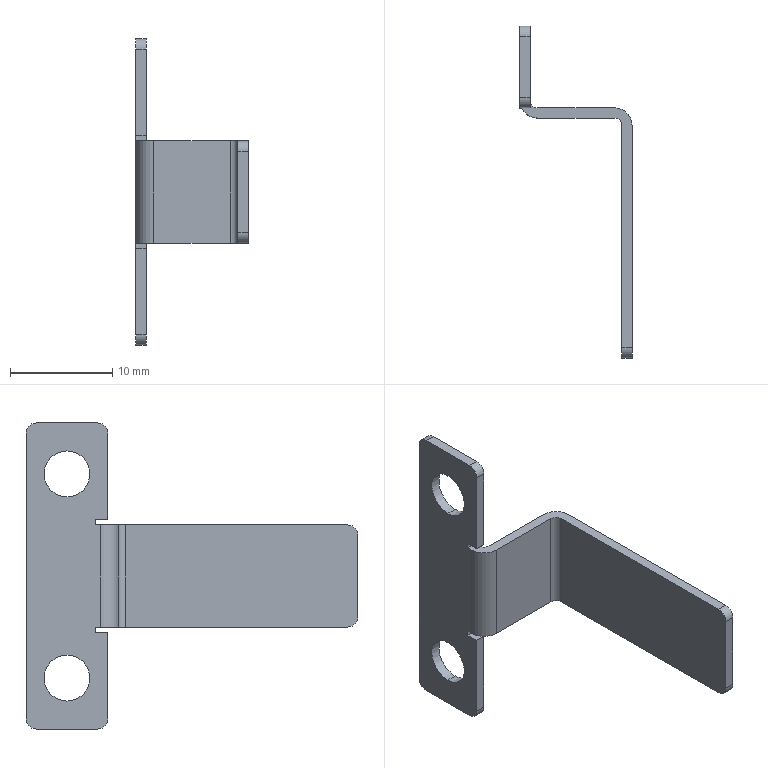Part | STEP file | 复件 FFH80-GY-019^复件 FFH85-PL-M75-B3-01_三轴模组 | 1 solid | 32 faces | box 11 x 32.5 x 30 mm | volume 540.052 mm3 | plane 18 | cylinder 14 | commonest cylinder face diameters 2 x6 4.5 x4 1.473 x2 3.473 x2
STEP:
#1=CARTESIAN_POINT('',(-1.,0.,-7.75));
#2=VERTEX_POINT('',#1);
#3=CARTESIAN_POINT('',(-1.,0.,-12.25));
#4=VERTEX_POINT('',#3);
#5=CARTESIAN_POINT('',(-1.,0.,-10.));
#6=DIRECTION('',(1.,0.,0.));
#7=DIRECTION('',(0.,0.,-1.));
#8=AXIS2_PLACEMENT_3D('',#5,#6,#7);
#9=CIRCLE('',#8,2.25);
#10=EDGE_CURVE('',#2,#4,#9,.T.);
#11=ORIENTED_EDGE('',*,*,#10,.F.);
#12=CARTESIAN_POINT('',(0.,0.,-7.75));
#13=VERTEX_POINT('',#12);
#14=CARTESIAN_POINT('',(0.,0.,-7.75));
#15=DIRECTION('',(1.,0.,0.));
#16=VECTOR('',#15,1000.);
#17=LINE('',#14,#16);
#18=EDGE_CURVE('',#2,#13,#17,.T.);
#19=ORIENTED_EDGE('',*,*,#18,.T.);
#20=CARTESIAN_POINT('',(0.,0.,-12.25));
#21=VERTEX_POINT('',#20);
#22=CARTESIAN_POINT('',(0.,0.,-10.));
#23=DIRECTION('',(1.,0.,0.));
#24=DIRECTION('',(0.,0.,-1.));
#25=AXIS2_PLACEMENT_3D('',#22,#23,#24);
#26=CIRCLE('',#25,2.25);
#27=EDGE_CURVE('',#13,#21,#26,.T.);
#28=ORIENTED_EDGE('',*,*,#27,.T.);
#29=CARTESIAN_POINT('',(0.,0.,-12.25));
#30=DIRECTION('',(1.,0.,0.));
#31=VECTOR('',#30,1000.);
#32=LINE('',#29,#31);
#33=EDGE_CURVE('',#4,#21,#32,.T.);
#34=ORIENTED_EDGE('',*,*,#33,.F.);
#35=EDGE_LOOP('',(#11,#19,#28,#34));
#36=FACE_OUTER_BOUND('',#35,.T.);
#37=CARTESIAN_POINT('',(0.,0.,-10.));
#38=DIRECTION('',(1.,0.,0.));
#39=DIRECTION('',(0.,0.,-1.));
#40=AXIS2_PLACEMENT_3D('',#37,#38,#39);
#41=CYLINDRICAL_SURFACE('',#40,2.25);
#42=ADVANCED_FACE('',(#36),#41,.F.);
#43=CARTESIAN_POINT('',(-1.,0.,12.25));
#44=VERTEX_POINT('',#43);
#45=CARTESIAN_POINT('',(-1.,0.,7.75));
#46=VERTEX_POINT('',#45);
#47=CARTESIAN_POINT('',(-1.,0.,10.));
#48=DIRECTION('',(1.,0.,0.));
#49=DIRECTION('',(0.,0.,-1.));
#50=AXIS2_PLACEMENT_3D('',#47,#48,#49);
#51=CIRCLE('',#50,2.25);
#52=EDGE_CURVE('',#44,#46,#51,.T.);
#53=ORIENTED_EDGE('',*,*,#52,.F.);
#54=CARTESIAN_POINT('',(0.,0.,12.25));
#55=VERTEX_POINT('',#54);
#56=CARTESIAN_POINT('',(0.,0.,12.25));
#57=DIRECTION('',(1.,0.,0.));
#58=VECTOR('',#57,1000.);
#59=LINE('',#56,#58);
#60=EDGE_CURVE('',#44,#55,#59,.T.);
#61=ORIENTED_EDGE('',*,*,#60,.T.);
#62=CARTESIAN_POINT('',(0.,0.,7.75));
#63=VERTEX_POINT('',#62);
#64=CARTESIAN_POINT('',(0.,0.,10.));
#65=DIRECTION('',(1.,0.,0.));
#66=DIRECTION('',(0.,0.,-1.));
#67=AXIS2_PLACEMENT_3D('',#64,#65,#66);
#68=CIRCLE('',#67,2.25);
#69=EDGE_CURVE('',#55,#63,#68,.T.);
#70=ORIENTED_EDGE('',*,*,#69,.T.);
#71=CARTESIAN_POINT('',(0.,0.,7.75));
#72=DIRECTION('',(1.,0.,0.));
#73=VECTOR('',#72,1000.);
#74=LINE('',#71,#73);
#75=EDGE_CURVE('',#46,#63,#74,.T.);
#76=ORIENTED_EDGE('',*,*,#75,.F.);
#77=EDGE_LOOP('',(#53,#61,#70,#76));
#78=FACE_OUTER_BOUND('',#77,.T.);
#79=CARTESIAN_POINT('',(0.,0.,10.));
#80=DIRECTION('',(1.,0.,0.));
#81=DIRECTION('',(0.,0.,-1.));
#82=AXIS2_PLACEMENT_3D('',#79,#80,#81);
#83=CYLINDRICAL_SURFACE('',#82,2.25);
#84=ADVANCED_FACE('',(#78),#83,.F.);
#85=CARTESIAN_POINT('',(9.,-27.5,5.));
#86=VERTEX_POINT('',#85);
#87=CARTESIAN_POINT('',(9.,-5.737,5.));
#88=VERTEX_POINT('',#87);
#89=CARTESIAN_POINT('',(9.,0.,5.));
#90=DIRECTION('',(0.,1.,0.));
#91=VECTOR('',#90,1000.);
#92=LINE('',#89,#91);
#93=EDGE_CURVE('',#86,#88,#92,.T.);
#94=ORIENTED_EDGE('',*,*,#93,.T.);
#95=CARTESIAN_POINT('',(9.,-5.737,-5.));
#96=VERTEX_POINT('',#95);
#97=CARTESIAN_POINT('',(9.,-5.737,0.));
#98=DIRECTION('',(0.,0.,-1.));
#99=VECTOR('',#98,1000.);
#100=LINE('',#97,#99);
#101=EDGE_CURVE('',#88,#96,#100,.T.);
#102=ORIENTED_EDGE('',*,*,#101,.T.);
#103=CARTESIAN_POINT('',(9.,-27.5,-5.));
#104=VERTEX_POINT('',#103);
#105=CARTESIAN_POINT('',(9.,0.,-5.));
#106=DIRECTION('',(0.,-1.,0.));
#107=VECTOR('',#106,1000.);
#108=LINE('',#105,#107);
#109=EDGE_CURVE('',#96,#104,#108,.T.);
#110=ORIENTED_EDGE('',*,*,#109,.T.);
#111=CARTESIAN_POINT('',(9.,-28.5,-4.));
#112=VERTEX_POINT('',#111);
#113=CARTESIAN_POINT('',(9.,-27.5,-4.));
#114=DIRECTION('',(-1.,0.,0.));
#115=DIRECTION('',(0.,-1.,0.));
#116=AXIS2_PLACEMENT_3D('',#113,#114,#115);
#117=CIRCLE('',#116,1.);
#118=EDGE_CURVE('',#104,#112,#117,.T.);
#119=ORIENTED_EDGE('',*,*,#118,.T.);
#120=CARTESIAN_POINT('',(9.,-28.5,4.));
#121=VERTEX_POINT('',#120);
#122=CARTESIAN_POINT('',(9.,-28.5,0.));
#123=DIRECTION('',(0.,0.,1.));
#124=VECTOR('',#123,1000.);
#125=LINE('',#122,#124);
#126=EDGE_CURVE('',#112,#121,#125,.T.);
#127=ORIENTED_EDGE('',*,*,#126,.T.);
#128=CARTESIAN_POINT('',(9.,-27.5,4.));
#129=DIRECTION('',(-1.,0.,0.));
#130=DIRECTION('',(0.,-1.,0.));
#131=AXIS2_PLACEMENT_3D('',#128,#129,#130);
#132=CIRCLE('',#131,1.);
#133=EDGE_CURVE('',#121,#86,#132,.T.);
#134=ORIENTED_EDGE('',*,*,#133,.T.);
#135=EDGE_LOOP('',(#94,#102,#110,#119,#127,#134));
#136=FACE_OUTER_BOUND('',#135,.T.);
#137=CARTESIAN_POINT('',(9.,0.,0.));
#138=DIRECTION('',(-1.,0.,0.));
#139=DIRECTION('',(0.,0.,1.));
#140=AXIS2_PLACEMENT_3D('',#137,#138,#139);
#141=PLANE('',#140);
#142=ADVANCED_FACE('',(#136),#141,.T.);
#143=ORIENTED_EDGE('',*,*,#101,.F.);
#144=CARTESIAN_POINT('',(8.263,-5.,5.));
#145=VERTEX_POINT('',#144);
#146=CARTESIAN_POINT('',(8.263,-5.737,5.));
#147=DIRECTION('',(0.,0.,-1.));
#148=DIRECTION('',(1.,0.,0.));
#149=AXIS2_PLACEMENT_3D('',#146,#147,#148);
#150=CIRCLE('',#149,0.7366);
#151=EDGE_CURVE('',#145,#88,#150,.T.);
#152=ORIENTED_EDGE('',*,*,#151,.F.);
#153=CARTESIAN_POINT('',(8.263,-5.,-5.));
#154=VERTEX_POINT('',#153);
#155=CARTESIAN_POINT('',(8.263,-5.,5.));
#156=DIRECTION('',(0.,0.,1.));
#157=VECTOR('',#156,1000.);
#158=LINE('',#155,#157);
#159=EDGE_CURVE('',#154,#145,#158,.T.);
#160=ORIENTED_EDGE('',*,*,#159,.F.);
#161=CARTESIAN_POINT('',(8.263,-5.737,-5.));
#162=DIRECTION('',(0.,0.,1.));
#163=DIRECTION('',(1.,0.,0.));
#164=AXIS2_PLACEMENT_3D('',#161,#162,#163);
#165=CIRCLE('',#164,0.7366);
#166=EDGE_CURVE('',#96,#154,#165,.T.);
#167=ORIENTED_EDGE('',*,*,#166,.F.);
#168=EDGE_LOOP('',(#143,#152,#160,#167));
#169=FACE_OUTER_BOUND('',#168,.T.);
#170=CARTESIAN_POINT('',(8.263,-5.737,5.));
#171=DIRECTION('',(0.,0.,1.));
#172=DIRECTION('',(1.,0.,0.));
#173=AXIS2_PLACEMENT_3D('',#170,#171,#172);
#174=CYLINDRICAL_SURFACE('',#173,0.7366);
#175=ADVANCED_FACE('',(#169),#174,.F.);
#176=CARTESIAN_POINT('',(10.,-5.737,5.));
#177=VERTEX_POINT('',#176);
#178=CARTESIAN_POINT('',(10.,-27.5,5.));
#179=VERTEX_POINT('',#178);
#180=CARTESIAN_POINT('',(10.,-28.5,5.));
#181=DIRECTION('',(0.,-1.,0.));
#182=VECTOR('',#181,1000.);
#183=LINE('',#180,#182);
#184=EDGE_CURVE('',#177,#179,#183,.T.);
#185=ORIENTED_EDGE('',*,*,#184,.F.);
#186=CARTESIAN_POINT('',(8.263,-4.,5.));
#187=VERTEX_POINT('',#186);
#188=CARTESIAN_POINT('',(8.263,-5.737,5.));
#189=DIRECTION('',(0.,0.,-1.));
#190=DIRECTION('',(1.,0.,0.));
#191=AXIS2_PLACEMENT_3D('',#188,#189,#190);
#192=CIRCLE('',#191,1.737);
#193=EDGE_CURVE('',#187,#177,#192,.T.);
#194=ORIENTED_EDGE('',*,*,#193,.F.);
#195=CARTESIAN_POINT('',(0.7366,-4.,5.));
#196=VERTEX_POINT('',#195);
#197=CARTESIAN_POINT('',(10.,-4.,5.));
#198=DIRECTION('',(1.,0.,0.));
#199=VECTOR('',#198,1000.);
#200=LINE('',#197,#199);
#201=EDGE_CURVE('',#196,#187,#200,.T.);
#202=ORIENTED_EDGE('',*,*,#201,.F.);
#203=CARTESIAN_POINT('',(0.,-3.263,5.));
#204=VERTEX_POINT('',#203);
#205=CARTESIAN_POINT('',(0.7366,-3.263,5.));
#206=DIRECTION('',(0.,0.,-1.));
#207=DIRECTION('',(0.,1.,0.));
#208=AXIS2_PLACEMENT_3D('',#205,#206,#207);
#209=CIRCLE('',#208,0.7366);
#210=EDGE_CURVE('',#196,#204,#209,.T.);
#211=ORIENTED_EDGE('',*,*,#210,.T.);
#212=CARTESIAN_POINT('',(0.,-2.763,5.));
#213=VERTEX_POINT('',#212);
#214=CARTESIAN_POINT('',(0.,0.,5.));
#215=DIRECTION('',(0.,1.,0.));
#216=VECTOR('',#215,1000.);
#217=LINE('',#214,#216);
#218=EDGE_CURVE('',#204,#213,#217,.T.);
#219=ORIENTED_EDGE('',*,*,#218,.T.);
#220=CARTESIAN_POINT('',(-1.,-2.763,5.));
#221=VERTEX_POINT('',#220);
#222=CARTESIAN_POINT('',(10.,-2.763,5.));
#223=DIRECTION('',(1.,0.,0.));
#224=VECTOR('',#223,1000.);
#225=LINE('',#222,#224);
#226=EDGE_CURVE('',#221,#213,#225,.T.);
#227=ORIENTED_EDGE('',*,*,#226,.F.);
#228=CARTESIAN_POINT('',(-1.,-3.263,5.));
#229=VERTEX_POINT('',#228);
#230=CARTESIAN_POINT('',(-1.,0.,5.));
#231=DIRECTION('',(0.,1.,0.));
#232=VECTOR('',#231,1000.);
#233=LINE('',#230,#232);
#234=EDGE_CURVE('',#229,#221,#233,.T.);
#235=ORIENTED_EDGE('',*,*,#234,.F.);
#236=CARTESIAN_POINT('',(0.7366,-5.,5.));
#237=VERTEX_POINT('',#236);
#238=CARTESIAN_POINT('',(0.7366,-3.263,5.));
#239=DIRECTION('',(0.,0.,-1.));
#240=DIRECTION('',(0.,1.,0.));
#241=AXIS2_PLACEMENT_3D('',#238,#239,#240);
#242=CIRCLE('',#241,1.737);
#243=EDGE_CURVE('',#237,#229,#242,.T.);
#244=ORIENTED_EDGE('',*,*,#243,.F.);
#245=CARTESIAN_POINT('',(10.,-5.,5.));
#246=DIRECTION('',(-1.,0.,0.));
#247=VECTOR('',#246,1000.);
#248=LINE('',#245,#247);
#249=EDGE_CURVE('',#145,#237,#248,.T.);
#250=ORIENTED_EDGE('',*,*,#249,.F.);
#251=ORIENTED_EDGE('',*,*,#151,.T.);
#252=ORIENTED_EDGE('',*,*,#93,.F.);
#253=CARTESIAN_POINT('',(10.,-27.5,5.));
#254=DIRECTION('',(-1.,0.,0.));
#255=VECTOR('',#254,1000.);
#256=LINE('',#253,#255);
#257=EDGE_CURVE('',#179,#86,#256,.T.);
#258=ORIENTED_EDGE('',*,*,#257,.F.);
#259=EDGE_LOOP('',(#185,#194,#202,#211,#219,#227,#235,#244,#250,#251,#252,#258));
#260=FACE_OUTER_BOUND('',#259,.T.);
#261=CARTESIAN_POINT('',(10.,-28.5,5.));
#262=DIRECTION('',(0.,0.,-1.));
#263=DIRECTION('',(0.,1.,0.));
#264=AXIS2_PLACEMENT_3D('',#261,#262,#263);
#265=PLANE('',#264);
#266=ADVANCED_FACE('',(#260),#265,.F.);
#267=CARTESIAN_POINT('',(10.,-28.5,4.));
#268=VERTEX_POINT('',#267);
#269=CARTESIAN_POINT('',(10.,-27.5,4.));
#270=DIRECTION('',(-1.,0.,0.));
#271=DIRECTION('',(0.,-1.,0.));
#272=AXIS2_PLACEMENT_3D('',#269,#270,#271);
#273=CIRCLE('',#272,1.);
#274=EDGE_CURVE('',#268,#179,#273,.T.);
#275=ORIENTED_EDGE('',*,*,#274,.T.);
#276=ORIENTED_EDGE('',*,*,#257,.T.);
#277=ORIENTED_EDGE('',*,*,#133,.F.);
#278=CARTESIAN_POINT('',(10.,-28.5,4.));
#279=DIRECTION('',(1.,0.,0.));
#280=VECTOR('',#279,1000.);
#281=LINE('',#278,#280);
#282=EDGE_CURVE('',#121,#268,#281,.T.);
#283=ORIENTED_EDGE('',*,*,#282,.T.);
#284=EDGE_LOOP('',(#275,#276,#277,#283));
#285=FACE_OUTER_BOUND('',#284,.T.);
#286=CARTESIAN_POINT('',(10.,-27.5,4.));
#287=DIRECTION('',(-1.,0.,0.));
#288=DIRECTION('',(0.,-1.,0.));
#289=AXIS2_PLACEMENT_3D('',#286,#287,#288);
#290=CYLINDRICAL_SURFACE('',#289,1.);
#291=ADVANCED_FACE('',(#285),#290,.T.);
#292=ORIENTED_EDGE('',*,*,#126,.F.);
#293=CARTESIAN_POINT('',(10.,-28.5,-4.));
#294=VERTEX_POINT('',#293);
#295=CARTESIAN_POINT('',(10.,-28.5,-4.));
#296=DIRECTION('',(-1.,0.,0.));
#297=VECTOR('',#296,1000.);
#298=LINE('',#295,#297);
#299=EDGE_CURVE('',#294,#112,#298,.T.);
#300=ORIENTED_EDGE('',*,*,#299,.F.);
#301=CARTESIAN_POINT('',(10.,-28.5,-5.));
#302=DIRECTION('',(0.,0.,-1.));
#303=VECTOR('',#302,1000.);
#304=LINE('',#301,#303);
#305=EDGE_CURVE('',#268,#294,#304,.T.);
#306=ORIENTED_EDGE('',*,*,#305,.F.);
#307=ORIENTED_EDGE('',*,*,#282,.F.);
#308=EDGE_LOOP('',(#292,#300,#306,#307));
#309=FACE_OUTER_BOUND('',#308,.T.);
#310=CARTESIAN_POINT('',(10.,-28.5,-5.));
#311=DIRECTION('',(0.,1.,0.));
#312=DIRECTION('',(-1.,0.,0.));
#313=AXIS2_PLACEMENT_3D('',#310,#311,#312);
#314=PLANE('',#313);
#315=ADVANCED_FACE('',(#309),#314,.F.);
#316=CARTESIAN_POINT('',(10.,-27.5,-5.));
#317=VERTEX_POINT('',#316);
#318=CARTESIAN_POINT('',(10.,-27.5,-4.));
#319=DIRECTION('',(-1.,0.,0.));
#320=DIRECTION('',(0.,-1.,0.));
#321=AXIS2_PLACEMENT_3D('',#318,#319,#320);
#322=CIRCLE('',#321,1.);
#323=EDGE_CURVE('',#317,#294,#322,.T.);
#324=ORIENTED_EDGE('',*,*,#323,.T.);
#325=ORIENTED_EDGE('',*,*,#299,.T.);
#326=ORIENTED_EDGE('',*,*,#118,.F.);
#327=CARTESIAN_POINT('',(10.,-27.5,-5.));
#328=DIRECTION('',(1.,0.,0.));
#329=VECTOR('',#328,1000.);
#330=LINE('',#327,#329);
#331=EDGE_CURVE('',#104,#317,#330,.T.);
#332=ORIENTED_EDGE('',*,*,#331,.T.);
#333=EDGE_LOOP('',(#324,#325,#326,#332));
#334=FACE_OUTER_BOUND('',#333,.T.);
#335=CARTESIAN_POINT('',(10.,-27.5,-4.));
#336=DIRECTION('',(-1.,0.,0.));
#337=DIRECTION('',(0.,-1.,0.));
#338=AXIS2_PLACEMENT_3D('',#335,#336,#337);
#339=CYLINDRICAL_SURFACE('',#338,1.);
#340=ADVANCED_FACE('',(#334),#339,.T.);
#341=ORIENTED_EDGE('',*,*,#109,.F.);
#342=ORIENTED_EDGE('',*,*,#166,.T.);
#343=CARTESIAN_POINT('',(0.7366,-5.,-5.));
#344=VERTEX_POINT('',#343);
#345=CARTESIAN_POINT('',(10.,-5.,-5.));
#346=DIRECTION('',(1.,0.,0.));
#347=VECTOR('',#346,1000.);
#348=LINE('',#345,#347);
#349=EDGE_CURVE('',#344,#154,#348,.T.);
#350=ORIENTED_EDGE('',*,*,#349,.F.);
#351=CARTESIAN_POINT('',(-1.,-3.263,-5.));
#352=VERTEX_POINT('',#351);
#353=CARTESIAN_POINT('',(0.7366,-3.263,-5.));
#354=DIRECTION('',(0.,0.,1.));
#355=DIRECTION('',(0.,1.,0.));
#356=AXIS2_PLACEMENT_3D('',#353,#354,#355);
#357=CIRCLE('',#356,1.737);
#358=EDGE_CURVE('',#352,#344,#357,.T.);
#359=ORIENTED_EDGE('',*,*,#358,.F.);
#360=CARTESIAN_POINT('',(-1.,-2.763,-5.));
#361=VERTEX_POINT('',#360);
#362=CARTESIAN_POINT('',(-1.,0.,-5.));
#363=DIRECTION('',(0.,-1.,0.));
#364=VECTOR('',#363,1000.);
#365=LINE('',#362,#364);
#366=EDGE_CURVE('',#361,#352,#365,.T.);
#367=ORIENTED_EDGE('',*,*,#366,.F.);
#368=CARTESIAN_POINT('',(0.,-2.763,-5.));
#369=VERTEX_POINT('',#368);
#370=CARTESIAN_POINT('',(10.,-2.763,-5.));
#371=DIRECTION('',(-1.,0.,0.));
#372=VECTOR('',#371,1000.);
#373=LINE('',#370,#372);
#374=EDGE_CURVE('',#369,#361,#373,.T.);
#375=ORIENTED_EDGE('',*,*,#374,.F.);
#376=CARTESIAN_POINT('',(0.,-3.263,-5.));
#377=VERTEX_POINT('',#376);
#378=CARTESIAN_POINT('',(0.,0.,-5.));
#379=DIRECTION('',(0.,-1.,0.));
#380=VECTOR('',#379,1000.);
#381=LINE('',#378,#380);
#382=EDGE_CURVE('',#369,#377,#381,.T.);
#383=ORIENTED_EDGE('',*,*,#382,.T.);
#384=CARTESIAN_POINT('',(0.7366,-4.,-5.));
#385=VERTEX_POINT('',#384);
#386=CARTESIAN_POINT('',(0.7366,-3.263,-5.));
#387=DIRECTION('',(0.,0.,1.));
#388=DIRECTION('',(0.,1.,0.));
#389=AXIS2_PLACEMENT_3D('',#386,#387,#388);
#390=CIRCLE('',#389,0.7366);
#391=EDGE_CURVE('',#377,#385,#390,.T.);
#392=ORIENTED_EDGE('',*,*,#391,.T.);
#393=CARTESIAN_POINT('',(8.263,-4.,-5.));
#394=VERTEX_POINT('',#393);
#395=CARTESIAN_POINT('',(10.,-4.,-5.));
#396=DIRECTION('',(-1.,0.,0.));
#397=VECTOR('',#396,1000.);
#398=LINE('',#395,#397);
#399=EDGE_CURVE('',#394,#385,#398,.T.);
#400=ORIENTED_EDGE('',*,*,#399,.F.);
#401=CARTESIAN_POINT('',(10.,-5.737,-5.));
#402=VERTEX_POINT('',#401);
#403=CARTESIAN_POINT('',(8.263,-5.737,-5.));
#404=DIRECTION('',(0.,0.,1.));
#405=DIRECTION('',(1.,0.,0.));
#406=AXIS2_PLACEMENT_3D('',#403,#404,#405);
#407=CIRCLE('',#406,1.737);
#408=EDGE_CURVE('',#402,#394,#407,.T.);
#409=ORIENTED_EDGE('',*,*,#408,.F.);
#410=CARTESIAN_POINT('',(10.,-5.,-5.));
#411=DIRECTION('',(0.,1.,0.));
#412=VECTOR('',#411,1000.);
#413=LINE('',#410,#412);
#414=EDGE_CURVE('',#317,#402,#413,.T.);
#415=ORIENTED_EDGE('',*,*,#414,.F.);
#416=ORIENTED_EDGE('',*,*,#331,.F.);
#417=EDGE_LOOP('',(#341,#342,#350,#359,#367,#375,#383,#392,#400,#409,#415,#416));
#418=FACE_OUTER_BOUND('',#417,.T.);
#419=CARTESIAN_POINT('',(10.,-5.,-5.));
#420=DIRECTION('',(0.,0.,1.));
#421=DIRECTION('',(0.,-1.,0.));
#422=AXIS2_PLACEMENT_3D('',#419,#420,#421);
#423=PLANE('',#422);
#424=ADVANCED_FACE('',(#418),#423,.F.);
#425=ORIENTED_EDGE('',*,*,#349,.T.);
#426=ORIENTED_EDGE('',*,*,#159,.T.);
#427=ORIENTED_EDGE('',*,*,#249,.T.);
#428=CARTESIAN_POINT('',(0.7366,-5.,0.));
#429=DIRECTION('',(0.,0.,-1.));
#430=VECTOR('',#429,1000.);
#431=LINE('',#428,#430);
#432=EDGE_CURVE('',#237,#344,#431,.T.);
#433=ORIENTED_EDGE('',*,*,#432,.T.);
#434=EDGE_LOOP('',(#425,#426,#427,#433));
#435=FACE_OUTER_BOUND('',#434,.T.);
#436=CARTESIAN_POINT('',(0.,-5.,0.));
#437=DIRECTION('',(0.,-1.,0.));
#438=DIRECTION('',(1.,0.,0.));
#439=AXIS2_PLACEMENT_3D('',#436,#437,#438);
#440=PLANE('',#439);
#441=ADVANCED_FACE('',(#435),#440,.T.);
#442=ORIENTED_EDGE('',*,*,#305,.T.);
#443=ORIENTED_EDGE('',*,*,#323,.F.);
#444=ORIENTED_EDGE('',*,*,#414,.T.);
#445=CARTESIAN_POINT('',(10.,-5.737,0.));
#446=DIRECTION('',(0.,0.,-1.));
#447=VECTOR('',#446,1000.);
#448=LINE('',#445,#447);
#449=EDGE_CURVE('',#177,#402,#448,.T.);
#450=ORIENTED_EDGE('',*,*,#449,.F.);
#451=ORIENTED_EDGE('',*,*,#184,.T.);
#452=ORIENTED_EDGE('',*,*,#274,.F.);
#453=EDGE_LOOP('',(#442,#443,#444,#450,#451,#452));
#454=FACE_OUTER_BOUND('',#453,.T.);
#455=CARTESIAN_POINT('',(10.,0.,0.));
#456=DIRECTION('',(-1.,0.,0.));
#457=DIRECTION('',(0.,0.,1.));
#458=AXIS2_PLACEMENT_3D('',#455,#456,#457);
#459=PLANE('',#458);
#460=ADVANCED_FACE('',(#454),#459,.F.);
#461=CARTESIAN_POINT('',(8.263,-4.,5.));
#462=DIRECTION('',(0.,0.,1.));
#463=VECTOR('',#462,1000.);
#464=LINE('',#461,#463);
#465=EDGE_CURVE('',#394,#187,#464,.T.);
#466=ORIENTED_EDGE('',*,*,#465,.T.);
#467=ORIENTED_EDGE('',*,*,#193,.T.);
#468=ORIENTED_EDGE('',*,*,#449,.T.);
#469=ORIENTED_EDGE('',*,*,#408,.T.);
#470=EDGE_LOOP('',(#466,#467,#468,#469));
#471=FACE_OUTER_BOUND('',#470,.T.);
#472=CARTESIAN_POINT('',(8.263,-5.737,5.));
#473=DIRECTION('',(0.,0.,1.));
#474=DIRECTION('',(1.,0.,0.));
#475=AXIS2_PLACEMENT_3D('',#472,#473,#474);
#476=CYLINDRICAL_SURFACE('',#475,1.737);
#477=ADVANCED_FACE('',(#471),#476,.T.);
#478=CARTESIAN_POINT('',(0.7366,-4.,0.));
#479=DIRECTION('',(0.,0.,-1.));
#480=VECTOR('',#479,1000.);
#481=LINE('',#478,#480);
#482=EDGE_CURVE('',#196,#385,#481,.T.);
#483=ORIENTED_EDGE('',*,*,#482,.F.);
#484=ORIENTED_EDGE('',*,*,#201,.T.);
#485=ORIENTED_EDGE('',*,*,#465,.F.);
#486=ORIENTED_EDGE('',*,*,#399,.T.);
#487=EDGE_LOOP('',(#483,#484,#485,#486));
#488=FACE_OUTER_BOUND('',#487,.T.);
#489=CARTESIAN_POINT('',(0.,-4.,0.));
#490=DIRECTION('',(0.,-1.,0.));
#491=DIRECTION('',(1.,0.,0.));
#492=AXIS2_PLACEMENT_3D('',#489,#490,#491);
#493=PLANE('',#492);
#494=ADVANCED_FACE('',(#488),#493,.F.);
#495=CARTESIAN_POINT('',(-1.,-2.763,5.5));
#496=VERTEX_POINT('',#495);
#497=CARTESIAN_POINT('',(-1.,-2.763,0.));
#498=DIRECTION('',(0.,0.,1.));
#499=VECTOR('',#498,1000.);
#500=LINE('',#497,#499);
#501=EDGE_CURVE('',#221,#496,#500,.T.);
#502=ORIENTED_EDGE('',*,*,#501,.F.);
#503=ORIENTED_EDGE('',*,*,#226,.T.);
#504=CARTESIAN_POINT('',(0.,-2.763,5.5));
#505=VERTEX_POINT('',#504);
#506=CARTESIAN_POINT('',(0.,-2.763,0.));
#507=DIRECTION('',(0.,0.,1.));
#508=VECTOR('',#507,1000.);
#509=LINE('',#506,#508);
#510=EDGE_CURVE('',#213,#505,#509,.T.);
#511=ORIENTED_EDGE('',*,*,#510,.T.);
#512=CARTESIAN_POINT('',(0.,-2.763,5.5));
#513=DIRECTION('',(-1.,0.,0.));
#514=VECTOR('',#513,1000.);
#515=LINE('',#512,#514);
#516=EDGE_CURVE('',#505,#496,#515,.T.);
#517=ORIENTED_EDGE('',*,*,#516,.T.);
#518=EDGE_LOOP('',(#502,#503,#511,#517));
#519=FACE_OUTER_BOUND('',#518,.T.);
#520=CARTESIAN_POINT('',(0.,-2.763,5.));
#521=DIRECTION('',(0.,-1.,0.));
#522=DIRECTION('',(0.,0.,-1.));
#523=AXIS2_PLACEMENT_3D('',#520,#521,#522);
#524=PLANE('',#523);
#525=ADVANCED_FACE('',(#519),#524,.T.);
#526=CARTESIAN_POINT('',(-1.,-3.263,-5.));
#527=DIRECTION('',(0.,0.,-1.));
#528=VECTOR('',#527,1000.);
#529=LINE('',#526,#528);
#530=EDGE_CURVE('',#229,#352,#529,.T.);
#531=ORIENTED_EDGE('',*,*,#530,.T.);
#532=ORIENTED_EDGE('',*,*,#358,.T.);
#533=ORIENTED_EDGE('',*,*,#432,.F.);
#534=ORIENTED_EDGE('',*,*,#243,.T.);
#535=EDGE_LOOP('',(#531,#532,#533,#534));
#536=FACE_OUTER_BOUND('',#535,.T.);
#537=CARTESIAN_POINT('',(0.7366,-3.263,-5.));
#538=DIRECTION('',(0.,0.,-1.));
#539=DIRECTION('',(0.,1.,0.));
#540=AXIS2_PLACEMENT_3D('',#537,#538,#539);
#541=CYLINDRICAL_SURFACE('',#540,1.737);
#542=ADVANCED_FACE('',(#536),#541,.T.);
#543=CARTESIAN_POINT('',(-1.,-2.763,-5.5));
#544=VERTEX_POINT('',#543);
#545=CARTESIAN_POINT('',(-1.,-2.763,-5.5));
#546=DIRECTION('',(0.,0.,-1.));
#547=VECTOR('',#546,1000.);
#548=LINE('',#545,#547);
#549=EDGE_CURVE('',#361,#544,#548,.T.);
#550=ORIENTED_EDGE('',*,*,#549,.T.);
#551=CARTESIAN_POINT('',(0.,-2.763,-5.5));
#552=VERTEX_POINT('',#551);
#553=CARTESIAN_POINT('',(0.,-2.763,-5.5));
#554=DIRECTION('',(1.,0.,0.));
#555=VECTOR('',#554,1000.);
#556=LINE('',#553,#555);
#557=EDGE_CURVE('',#544,#552,#556,.T.);
#558=ORIENTED_EDGE('',*,*,#557,.T.);
#559=CARTESIAN_POINT('',(0.,-2.763,0.));
#560=DIRECTION('',(0.,0.,1.));
#561=VECTOR('',#560,1000.);
#562=LINE('',#559,#561);
#563=EDGE_CURVE('',#552,#369,#562,.T.);
#564=ORIENTED_EDGE('',*,*,#563,.T.);
#565=ORIENTED_EDGE('',*,*,#374,.T.);
#566=EDGE_LOOP('',(#550,#558,#564,#565));
#567=FACE_OUTER_BOUND('',#566,.T.);
#568=CARTESIAN_POINT('',(0.,-2.763,-5.5));
#569=DIRECTION('',(0.,-1.,0.));
#570=DIRECTION('',(0.,0.,-1.));
#571=AXIS2_PLACEMENT_3D('',#568,#569,#570);
#572=PLANE('',#571);
#573=ADVANCED_FACE('',(#567),#572,.T.);
#574=ORIENTED_EDGE('',*,*,#482,.T.);
#575=ORIENTED_EDGE('',*,*,#391,.F.);
#576=CARTESIAN_POINT('',(0.,-3.263,-5.));
#577=DIRECTION('',(0.,0.,-1.));
#578=VECTOR('',#577,1000.);
#579=LINE('',#576,#578);
#580=EDGE_CURVE('',#204,#377,#579,.T.);
#581=ORIENTED_EDGE('',*,*,#580,.F.);
#582=ORIENTED_EDGE('',*,*,#210,.F.);
#583=EDGE_LOOP('',(#574,#575,#581,#582));
#584=FACE_OUTER_BOUND('',#583,.T.);
#585=CARTESIAN_POINT('',(0.7366,-3.263,-5.));
#586=DIRECTION('',(0.,0.,-1.));
#587=DIRECTION('',(0.,1.,0.));
#588=AXIS2_PLACEMENT_3D('',#585,#586,#587);
#589=CYLINDRICAL_SURFACE('',#588,0.7366);
#590=ADVANCED_FACE('',(#584),#589,.F.);
#591=CARTESIAN_POINT('',(-1.,-4.,5.5));
#592=VERTEX_POINT('',#591);
#593=CARTESIAN_POINT('',(-1.,-2.763,5.5));
#594=DIRECTION('',(0.,1.,0.));
#595=VECTOR('',#594,1000.);
#596=LINE('',#593,#595);
#597=EDGE_CURVE('',#592,#496,#596,.T.);
#598=ORIENTED_EDGE('',*,*,#597,.T.);
#599=ORIENTED_EDGE('',*,*,#516,.F.);
#600=CARTESIAN_POINT('',(0.,-4.,5.5));
#601=VERTEX_POINT('',#600);
#602=CARTESIAN_POINT('',(0.,-2.763,5.5));
#603=DIRECTION('',(0.,-1.,0.));
#604=VECTOR('',#603,1000.);
#605=LINE('',#602,#604);
#606=EDGE_CURVE('',#505,#601,#605,.T.);
#607=ORIENTED_EDGE('',*,*,#606,.T.);
#608=CARTESIAN_POINT('',(-1.,-4.,5.5));
#609=DIRECTION('',(1.,0.,0.));
#610=VECTOR('',#609,1000.);
#611=LINE('',#608,#610);
#612=EDGE_CURVE('',#592,#601,#611,.T.);
#613=ORIENTED_EDGE('',*,*,#612,.F.);
#614=EDGE_LOOP('',(#598,#599,#607,#613));
#615=FACE_OUTER_BOUND('',#614,.T.);
#616=CARTESIAN_POINT('',(0.,-2.763,5.5));
#617=DIRECTION('',(0.,0.,-1.));
#618=DIRECTION('',(-1.,0.,0.));
#619=AXIS2_PLACEMENT_3D('',#616,#617,#618);
#620=PLANE('',#619);
#621=ADVANCED_FACE('',(#615),#620,.T.);
#622=CARTESIAN_POINT('',(-1.,0.,-10.));
#623=DIRECTION('',(1.,0.,0.));
#624=DIRECTION('',(0.,0.,-1.));
#625=AXIS2_PLACEMENT_3D('',#622,#623,#624);
#626=CIRCLE('',#625,2.25);
#627=EDGE_CURVE('',#4,#2,#626,.T.);
#628=ORIENTED_EDGE('',*,*,#627,.T.);
#629=ORIENTED_EDGE('',*,*,#10,.T.);
#630=EDGE_LOOP('',(#628,#629));
#631=FACE_BOUND('',#630,.T.);
#632=CARTESIAN_POINT('',(-1.,0.,10.));
#633=DIRECTION('',(1.,0.,0.));
#634=DIRECTION('',(0.,0.,-1.));
#635=AXIS2_PLACEMENT_3D('',#632,#633,#634);
#636=CIRCLE('',#635,2.25);
#637=EDGE_CURVE('',#46,#44,#636,.T.);
#638=ORIENTED_EDGE('',*,*,#637,.T.);
#639=ORIENTED_EDGE('',*,*,#52,.T.);
#640=EDGE_LOOP('',(#638,#639));
#641=FACE_BOUND('',#640,.T.);
#642=CARTESIAN_POINT('',(-1.,-3.,15.));
#643=VERTEX_POINT('',#642);
#644=CARTESIAN_POINT('',(-1.,3.,15.));
#645=VERTEX_POINT('',#644);
#646=CARTESIAN_POINT('',(-1.,0.,15.));
#647=DIRECTION('',(0.,1.,0.));
#648=VECTOR('',#647,1000.);
#649=LINE('',#646,#648);
#650=EDGE_CURVE('',#643,#645,#649,.T.);
#651=ORIENTED_EDGE('',*,*,#650,.T.);
#652=CARTESIAN_POINT('',(-1.,4.,14.));
#653=VERTEX_POINT('',#652);
#654=CARTESIAN_POINT('',(-1.,3.,14.));
#655=DIRECTION('',(-1.,0.,0.));
#656=DIRECTION('',(0.,0.,-1.));
#657=AXIS2_PLACEMENT_3D('',#654,#655,#656);
#658=CIRCLE('',#657,1.);
#659=EDGE_CURVE('',#645,#653,#658,.T.);
#660=ORIENTED_EDGE('',*,*,#659,.T.);
#661=CARTESIAN_POINT('',(-1.,4.,-14.));
#662=VERTEX_POINT('',#661);
#663=CARTESIAN_POINT('',(-1.,4.,0.));
#664=DIRECTION('',(0.,0.,-1.));
#665=VECTOR('',#664,1000.);
#666=LINE('',#663,#665);
#667=EDGE_CURVE('',#653,#662,#666,.T.);
#668=ORIENTED_EDGE('',*,*,#667,.T.);
#669=CARTESIAN_POINT('',(-1.,3.,-15.));
#670=VERTEX_POINT('',#669);
#671=CARTESIAN_POINT('',(-1.,3.,-14.));
#672=DIRECTION('',(-1.,0.,0.));
#673=DIRECTION('',(0.,0.,-1.));
#674=AXIS2_PLACEMENT_3D('',#671,#672,#673);
#675=CIRCLE('',#674,1.);
#676=EDGE_CURVE('',#662,#670,#675,.T.);
#677=ORIENTED_EDGE('',*,*,#676,.T.);
#678=CARTESIAN_POINT('',(-1.,-3.,-15.));
#679=VERTEX_POINT('',#678);
#680=CARTESIAN_POINT('',(-1.,0.,-15.));
#681=DIRECTION('',(0.,-1.,0.));
#682=VECTOR('',#681,1000.);
#683=LINE('',#680,#682);
#684=EDGE_CURVE('',#670,#679,#683,.T.);
#685=ORIENTED_EDGE('',*,*,#684,.T.);
#686=CARTESIAN_POINT('',(-1.,-4.,-14.));
#687=VERTEX_POINT('',#686);
#688=CARTESIAN_POINT('',(-1.,-3.,-14.));
#689=DIRECTION('',(-1.,0.,0.));
#690=DIRECTION('',(0.,0.,-1.));
#691=AXIS2_PLACEMENT_3D('',#688,#689,#690);
#692=CIRCLE('',#691,1.);
#693=EDGE_CURVE('',#679,#687,#692,.T.);
#694=ORIENTED_EDGE('',*,*,#693,.T.);
#695=CARTESIAN_POINT('',(-1.,-4.,-5.5));
#696=VERTEX_POINT('',#695);
#697=CARTESIAN_POINT('',(-1.,-4.,0.));
#698=DIRECTION('',(0.,0.,1.));
#699=VECTOR('',#698,1000.);
#700=LINE('',#697,#699);
#701=EDGE_CURVE('',#687,#696,#700,.T.);
#702=ORIENTED_EDGE('',*,*,#701,.T.);
#703=CARTESIAN_POINT('',(-1.,0.,-5.5));
#704=DIRECTION('',(0.,1.,0.));
#705=VECTOR('',#704,1000.);
#706=LINE('',#703,#705);
#707=EDGE_CURVE('',#696,#544,#706,.T.);
#708=ORIENTED_EDGE('',*,*,#707,.T.);
#709=ORIENTED_EDGE('',*,*,#549,.F.);
#710=ORIENTED_EDGE('',*,*,#366,.T.);
#711=ORIENTED_EDGE('',*,*,#530,.F.);
#712=ORIENTED_EDGE('',*,*,#234,.T.);
#713=ORIENTED_EDGE('',*,*,#501,.T.);
#714=ORIENTED_EDGE('',*,*,#597,.F.);
#715=CARTESIAN_POINT('',(-1.,-4.,14.));
#716=VERTEX_POINT('',#715);
#717=CARTESIAN_POINT('',(-1.,-4.,0.));
#718=DIRECTION('',(0.,0.,1.));
#719=VECTOR('',#718,1000.);
#720=LINE('',#717,#719);
#721=EDGE_CURVE('',#592,#716,#720,.T.);
#722=ORIENTED_EDGE('',*,*,#721,.T.);
#723=CARTESIAN_POINT('',(-1.,-3.,14.));
#724=DIRECTION('',(-1.,0.,0.));
#725=DIRECTION('',(0.,0.,-1.));
#726=AXIS2_PLACEMENT_3D('',#723,#724,#725);
#727=CIRCLE('',#726,1.);
#728=EDGE_CURVE('',#716,#643,#727,.T.);
#729=ORIENTED_EDGE('',*,*,#728,.T.);
#730=EDGE_LOOP('',(#651,#660,#668,#677,#685,#694,#702,#708,#709,#710,#711,#712,#713,#714,#722,#729));
#731=FACE_OUTER_BOUND('',#730,.T.);
#732=CARTESIAN_POINT('',(-1.,0.,0.));
#733=DIRECTION('',(-1.,0.,0.));
#734=DIRECTION('',(0.,0.,1.));
#735=AXIS2_PLACEMENT_3D('',#732,#733,#734);
#736=PLANE('',#735);
#737=ADVANCED_FACE('',(#631,#641,#731),#736,.T.);
#738=ORIENTED_EDGE('',*,*,#707,.F.);
#739=CARTESIAN_POINT('',(0.,-4.,-5.5));
#740=VERTEX_POINT('',#739);
#741=CARTESIAN_POINT('',(0.,-4.,-5.5));
#742=DIRECTION('',(1.,0.,0.));
#743=VECTOR('',#742,1000.);
#744=LINE('',#741,#743);
#745=EDGE_CURVE('',#696,#740,#744,.T.);
#746=ORIENTED_EDGE('',*,*,#745,.T.);
#747=CARTESIAN_POINT('',(0.,-4.,-5.5));
#748=DIRECTION('',(0.,1.,0.));
#749=VECTOR('',#748,1000.);
#750=LINE('',#747,#749);
#751=EDGE_CURVE('',#740,#552,#750,.T.);
#752=ORIENTED_EDGE('',*,*,#751,.T.);
#753=ORIENTED_EDGE('',*,*,#557,.F.);
#754=EDGE_LOOP('',(#738,#746,#752,#753));
#755=FACE_OUTER_BOUND('',#754,.T.);
#756=CARTESIAN_POINT('',(0.,-4.,-5.5));
#757=DIRECTION('',(0.,0.,1.));
#758=DIRECTION('',(1.,0.,0.));
#759=AXIS2_PLACEMENT_3D('',#756,#757,#758);
#760=PLANE('',#759);
#761=ADVANCED_FACE('',(#755),#760,.T.);
#762=CARTESIAN_POINT('',(0.,0.,-10.));
#763=DIRECTION('',(1.,0.,0.));
#764=DIRECTION('',(0.,0.,-1.));
#765=AXIS2_PLACEMENT_3D('',#762,#763,#764);
#766=CIRCLE('',#765,2.25);
#767=EDGE_CURVE('',#21,#13,#766,.T.);
#768=ORIENTED_EDGE('',*,*,#767,.F.);
#769=ORIENTED_EDGE('',*,*,#27,.F.);
#770=EDGE_LOOP('',(#768,#769));
#771=FACE_BOUND('',#770,.T.);
#772=CARTESIAN_POINT('',(0.,0.,10.));
#773=DIRECTION('',(1.,0.,0.));
#774=DIRECTION('',(0.,0.,-1.));
#775=AXIS2_PLACEMENT_3D('',#772,#773,#774);
#776=CIRCLE('',#775,2.25);
#777=EDGE_CURVE('',#63,#55,#776,.T.);
#778=ORIENTED_EDGE('',*,*,#777,.F.);
#779=ORIENTED_EDGE('',*,*,#69,.F.);
#780=EDGE_LOOP('',(#778,#779));
#781=FACE_BOUND('',#780,.T.);
#782=CARTESIAN_POINT('',(0.,3.,-15.));
#783=VERTEX_POINT('',#782);
#784=CARTESIAN_POINT('',(0.,-3.,-15.));
#785=VERTEX_POINT('',#784);
#786=CARTESIAN_POINT('',(0.,0.,-15.));
#787=DIRECTION('',(0.,-1.,0.));
#788=VECTOR('',#787,1000.);
#789=LINE('',#786,#788);
#790=EDGE_CURVE('',#783,#785,#789,.T.);
#791=ORIENTED_EDGE('',*,*,#790,.F.);
#792=CARTESIAN_POINT('',(0.,4.,-14.));
#793=VERTEX_POINT('',#792);
#794=CARTESIAN_POINT('',(0.,3.,-14.));
#795=DIRECTION('',(-1.,0.,0.));
#796=DIRECTION('',(0.,0.,-1.));
#797=AXIS2_PLACEMENT_3D('',#794,#795,#796);
#798=CIRCLE('',#797,1.);
#799=EDGE_CURVE('',#793,#783,#798,.T.);
#800=ORIENTED_EDGE('',*,*,#799,.F.);
#801=CARTESIAN_POINT('',(0.,4.,14.));
#802=VERTEX_POINT('',#801);
#803=CARTESIAN_POINT('',(0.,4.,0.));
#804=DIRECTION('',(0.,0.,-1.));
#805=VECTOR('',#804,1000.);
#806=LINE('',#803,#805);
#807=EDGE_CURVE('',#802,#793,#806,.T.);
#808=ORIENTED_EDGE('',*,*,#807,.F.);
#809=CARTESIAN_POINT('',(0.,3.,15.));
#810=VERTEX_POINT('',#809);
#811=CARTESIAN_POINT('',(0.,3.,14.));
#812=DIRECTION('',(-1.,0.,0.));
#813=DIRECTION('',(0.,0.,-1.));
#814=AXIS2_PLACEMENT_3D('',#811,#812,#813);
#815=CIRCLE('',#814,1.);
#816=EDGE_CURVE('',#810,#802,#815,.T.);
#817=ORIENTED_EDGE('',*,*,#816,.F.);
#818=CARTESIAN_POINT('',(0.,-3.,15.));
#819=VERTEX_POINT('',#818);
#820=CARTESIAN_POINT('',(0.,0.,15.));
#821=DIRECTION('',(0.,1.,0.));
#822=VECTOR('',#821,1000.);
#823=LINE('',#820,#822);
#824=EDGE_CURVE('',#819,#810,#823,.T.);
#825=ORIENTED_EDGE('',*,*,#824,.F.);
#826=CARTESIAN_POINT('',(0.,-4.,14.));
#827=VERTEX_POINT('',#826);
#828=CARTESIAN_POINT('',(0.,-3.,14.));
#829=DIRECTION('',(-1.,0.,0.));
#830=DIRECTION('',(0.,0.,-1.));
#831=AXIS2_PLACEMENT_3D('',#828,#829,#830);
#832=CIRCLE('',#831,1.);
#833=EDGE_CURVE('',#827,#819,#832,.T.);
#834=ORIENTED_EDGE('',*,*,#833,.F.);
#835=CARTESIAN_POINT('',(0.,-4.,0.));
#836=DIRECTION('',(0.,0.,1.));
#837=VECTOR('',#836,1000.);
#838=LINE('',#835,#837);
#839=EDGE_CURVE('',#601,#827,#838,.T.);
#840=ORIENTED_EDGE('',*,*,#839,.F.);
#841=ORIENTED_EDGE('',*,*,#606,.F.);
#842=ORIENTED_EDGE('',*,*,#510,.F.);
#843=ORIENTED_EDGE('',*,*,#218,.F.);
#844=ORIENTED_EDGE('',*,*,#580,.T.);
#845=ORIENTED_EDGE('',*,*,#382,.F.);
#846=ORIENTED_EDGE('',*,*,#563,.F.);
#847=ORIENTED_EDGE('',*,*,#751,.F.);
#848=CARTESIAN_POINT('',(0.,-4.,-14.));
#849=VERTEX_POINT('',#848);
#850=CARTESIAN_POINT('',(0.,-4.,0.));
#851=DIRECTION('',(0.,0.,1.));
#852=VECTOR('',#851,1000.);
#853=LINE('',#850,#852);
#854=EDGE_CURVE('',#849,#740,#853,.T.);
#855=ORIENTED_EDGE('',*,*,#854,.F.);
#856=CARTESIAN_POINT('',(0.,-3.,-14.));
#857=DIRECTION('',(-1.,0.,0.));
#858=DIRECTION('',(0.,0.,-1.));
#859=AXIS2_PLACEMENT_3D('',#856,#857,#858);
#860=CIRCLE('',#859,1.);
#861=EDGE_CURVE('',#785,#849,#860,.T.);
#862=ORIENTED_EDGE('',*,*,#861,.F.);
#863=EDGE_LOOP('',(#791,#800,#808,#817,#825,#834,#840,#841,#842,#843,#844,#845,#846,#847,#855,#862));
#864=FACE_OUTER_BOUND('',#863,.T.);
#865=CARTESIAN_POINT('',(0.,0.,0.));
#866=DIRECTION('',(-1.,0.,0.));
#867=DIRECTION('',(0.,0.,1.));
#868=AXIS2_PLACEMENT_3D('',#865,#866,#867);
#869=PLANE('',#868);
#870=ADVANCED_FACE('',(#771,#781,#864),#869,.F.);
#871=ORIENTED_EDGE('',*,*,#18,.F.);
#872=ORIENTED_EDGE('',*,*,#627,.F.);
#873=ORIENTED_EDGE('',*,*,#33,.T.);
#874=ORIENTED_EDGE('',*,*,#767,.T.);
#875=EDGE_LOOP('',(#871,#872,#873,#874));
#876=FACE_OUTER_BOUND('',#875,.T.);
#877=CARTESIAN_POINT('',(0.,0.,-10.));
#878=DIRECTION('',(1.,0.,0.));
#879=DIRECTION('',(0.,0.,-1.));
#880=AXIS2_PLACEMENT_3D('',#877,#878,#879);
#881=CYLINDRICAL_SURFACE('',#880,2.25);
#882=ADVANCED_FACE('',(#876),#881,.F.);
#883=ORIENTED_EDGE('',*,*,#60,.F.);
#884=ORIENTED_EDGE('',*,*,#637,.F.);
#885=ORIENTED_EDGE('',*,*,#75,.T.);
#886=ORIENTED_EDGE('',*,*,#777,.T.);
#887=EDGE_LOOP('',(#883,#884,#885,#886));
#888=FACE_OUTER_BOUND('',#887,.T.);
#889=CARTESIAN_POINT('',(0.,0.,10.));
#890=DIRECTION('',(1.,0.,0.));
#891=DIRECTION('',(0.,0.,-1.));
#892=AXIS2_PLACEMENT_3D('',#889,#890,#891);
#893=CYLINDRICAL_SURFACE('',#892,2.25);
#894=ADVANCED_FACE('',(#888),#893,.F.);
#895=ORIENTED_EDGE('',*,*,#659,.F.);
#896=CARTESIAN_POINT('',(-1.,3.,15.));
#897=DIRECTION('',(1.,0.,0.));
#898=VECTOR('',#897,1000.);
#899=LINE('',#896,#898);
#900=EDGE_CURVE('',#645,#810,#899,.T.);
#901=ORIENTED_EDGE('',*,*,#900,.T.);
#902=ORIENTED_EDGE('',*,*,#816,.T.);
#903=CARTESIAN_POINT('',(-1.,4.,14.));
#904=DIRECTION('',(-1.,0.,0.));
#905=VECTOR('',#904,1000.);
#906=LINE('',#903,#905);
#907=EDGE_CURVE('',#802,#653,#906,.T.);
#908=ORIENTED_EDGE('',*,*,#907,.T.);
#909=EDGE_LOOP('',(#895,#901,#902,#908));
#910=FACE_OUTER_BOUND('',#909,.T.);
#911=CARTESIAN_POINT('',(-1.,3.,14.));
#912=DIRECTION('',(1.,0.,0.));
#913=DIRECTION('',(0.,0.,-1.));
#914=AXIS2_PLACEMENT_3D('',#911,#912,#913);
#915=CYLINDRICAL_SURFACE('',#914,1.);
#916=ADVANCED_FACE('',(#910),#915,.T.);
#917=ORIENTED_EDGE('',*,*,#650,.F.);
#918=CARTESIAN_POINT('',(-1.,-3.,15.));
#919=DIRECTION('',(1.,0.,0.));
#920=VECTOR('',#919,1000.);
#921=LINE('',#918,#920);
#922=EDGE_CURVE('',#643,#819,#921,.T.);
#923=ORIENTED_EDGE('',*,*,#922,.T.);
#924=ORIENTED_EDGE('',*,*,#824,.T.);
#925=ORIENTED_EDGE('',*,*,#900,.F.);
#926=EDGE_LOOP('',(#917,#923,#924,#925));
#927=FACE_OUTER_BOUND('',#926,.T.);
#928=CARTESIAN_POINT('',(-1.,4.,15.));
#929=DIRECTION('',(0.,0.,1.));
#930=DIRECTION('',(0.,-1.,0.));
#931=AXIS2_PLACEMENT_3D('',#928,#929,#930);
#932=PLANE('',#931);
#933=ADVANCED_FACE('',(#927),#932,.T.);
#934=ORIENTED_EDGE('',*,*,#728,.F.);
#935=CARTESIAN_POINT('',(-1.,-4.,14.));
#936=DIRECTION('',(1.,0.,0.));
#937=VECTOR('',#936,1000.);
#938=LINE('',#935,#937);
#939=EDGE_CURVE('',#716,#827,#938,.T.);
#940=ORIENTED_EDGE('',*,*,#939,.T.);
#941=ORIENTED_EDGE('',*,*,#833,.T.);
#942=ORIENTED_EDGE('',*,*,#922,.F.);
#943=EDGE_LOOP('',(#934,#940,#941,#942));
#944=FACE_OUTER_BOUND('',#943,.T.);
#945=CARTESIAN_POINT('',(-1.,-3.,14.));
#946=DIRECTION('',(1.,0.,0.));
#947=DIRECTION('',(0.,0.,-1.));
#948=AXIS2_PLACEMENT_3D('',#945,#946,#947);
#949=CYLINDRICAL_SURFACE('',#948,1.);
#950=ADVANCED_FACE('',(#944),#949,.T.);
#951=ORIENTED_EDGE('',*,*,#839,.T.);
#952=ORIENTED_EDGE('',*,*,#939,.F.);
#953=ORIENTED_EDGE('',*,*,#721,.F.);
#954=ORIENTED_EDGE('',*,*,#612,.T.);
#955=EDGE_LOOP('',(#951,#952,#953,#954));
#956=FACE_OUTER_BOUND('',#955,.T.);
#957=CARTESIAN_POINT('',(-1.,-4.,-15.));
#958=DIRECTION('',(0.,-1.,0.));
#959=DIRECTION('',(0.,0.,-1.));
#960=AXIS2_PLACEMENT_3D('',#957,#958,#959);
#961=PLANE('',#960);
#962=ADVANCED_FACE('',(#956),#961,.T.);
#963=ORIENTED_EDGE('',*,*,#701,.F.);
#964=CARTESIAN_POINT('',(-1.,-4.,-14.));
#965=DIRECTION('',(1.,0.,0.));
#966=VECTOR('',#965,1000.);
#967=LINE('',#964,#966);
#968=EDGE_CURVE('',#687,#849,#967,.T.);
#969=ORIENTED_EDGE('',*,*,#968,.T.);
#970=ORIENTED_EDGE('',*,*,#854,.T.);
#971=ORIENTED_EDGE('',*,*,#745,.F.);
#972=EDGE_LOOP('',(#963,#969,#970,#971));
#973=FACE_OUTER_BOUND('',#972,.T.);
#974=CARTESIAN_POINT('',(-1.,-4.,-15.));
#975=DIRECTION('',(0.,-1.,0.));
#976=DIRECTION('',(0.,0.,-1.));
#977=AXIS2_PLACEMENT_3D('',#974,#975,#976);
#978=PLANE('',#977);
#979=ADVANCED_FACE('',(#973),#978,.T.);
#980=ORIENTED_EDGE('',*,*,#693,.F.);
#981=CARTESIAN_POINT('',(-1.,-3.,-15.));
#982=DIRECTION('',(1.,0.,0.));
#983=VECTOR('',#982,1000.);
#984=LINE('',#981,#983);
#985=EDGE_CURVE('',#679,#785,#984,.T.);
#986=ORIENTED_EDGE('',*,*,#985,.T.);
#987=ORIENTED_EDGE('',*,*,#861,.T.);
#988=ORIENTED_EDGE('',*,*,#968,.F.);
#989=EDGE_LOOP('',(#980,#986,#987,#988));
#990=FACE_OUTER_BOUND('',#989,.T.);
#991=CARTESIAN_POINT('',(-1.,-3.,-14.));
#992=DIRECTION('',(1.,0.,0.));
#993=DIRECTION('',(0.,0.,-1.));
#994=AXIS2_PLACEMENT_3D('',#991,#992,#993);
#995=CYLINDRICAL_SURFACE('',#994,1.);
#996=ADVANCED_FACE('',(#990),#995,.T.);
#997=ORIENTED_EDGE('',*,*,#790,.T.);
#998=ORIENTED_EDGE('',*,*,#985,.F.);
#999=ORIENTED_EDGE('',*,*,#684,.F.);
#1000=CARTESIAN_POINT('',(-1.,3.,-15.));
#1001=DIRECTION('',(1.,0.,0.));
#1002=VECTOR('',#1001,1000.);
#1003=LINE('',#1000,#1002);
#1004=EDGE_CURVE('',#670,#783,#1003,.T.);
#1005=ORIENTED_EDGE('',*,*,#1004,.T.);
#1006=EDGE_LOOP('',(#997,#998,#999,#1005));
#1007=FACE_OUTER_BOUND('',#1006,.T.);
#1008=CARTESIAN_POINT('',(-1.,4.,-15.));
#1009=DIRECTION('',(0.,0.,-1.));
#1010=DIRECTION('',(0.,1.,0.));
#1011=AXIS2_PLACEMENT_3D('',#1008,#1009,#1010);
#1012=PLANE('',#1011);
#1013=ADVANCED_FACE('',(#1007),#1012,.T.);
#1014=ORIENTED_EDGE('',*,*,#676,.F.);
#1015=CARTESIAN_POINT('',(-1.,4.,-14.));
#1016=DIRECTION('',(1.,0.,0.));
#1017=VECTOR('',#1016,1000.);
#1018=LINE('',#1015,#1017);
#1019=EDGE_CURVE('',#662,#793,#1018,.T.);
#1020=ORIENTED_EDGE('',*,*,#1019,.T.);
#1021=ORIENTED_EDGE('',*,*,#799,.T.);
#1022=ORIENTED_EDGE('',*,*,#1004,.F.);
#1023=EDGE_LOOP('',(#1014,#1020,#1021,#1022));
#1024=FACE_OUTER_BOUND('',#1023,.T.);
#1025=CARTESIAN_POINT('',(-1.,3.,-14.));
#1026=DIRECTION('',(1.,0.,0.));
#1027=DIRECTION('',(0.,0.,-1.));
#1028=AXIS2_PLACEMENT_3D('',#1025,#1026,#1027);
#1029=CYLINDRICAL_SURFACE('',#1028,1.);
#1030=ADVANCED_FACE('',(#1024),#1029,.T.);
#1031=ORIENTED_EDGE('',*,*,#807,.T.);
#1032=ORIENTED_EDGE('',*,*,#1019,.F.);
#1033=ORIENTED_EDGE('',*,*,#667,.F.);
#1034=ORIENTED_EDGE('',*,*,#907,.F.);
#1035=EDGE_LOOP('',(#1031,#1032,#1033,#1034));
#1036=FACE_OUTER_BOUND('',#1035,.T.);
#1037=CARTESIAN_POINT('',(-1.,4.,-15.));
#1038=DIRECTION('',(0.,1.,0.));
#1039=DIRECTION('',(0.,0.,1.));
#1040=AXIS2_PLACEMENT_3D('',#1037,#1038,#1039);
#1041=PLANE('',#1040);
#1042=ADVANCED_FACE('',(#1036),#1041,.T.);
#1043=CLOSED_SHELL('',(#42,#84,#142,#175,#266,#291,#315,#340,#424,#441,#460,#477,#494,#525,#542,#573,#590,#621,#737,#761,#870,#882,#894,#916,#933,#950,#962,#979,#996,#1013,#1030,#1042));
#1044=MANIFOLD_SOLID_BREP('',#1043);
#1045=CARTESIAN_POINT('',(0.,0.,0.));
#1046=DIRECTION('',(0.,0.,1.));
#1047=DIRECTION('',(1.,0.,0.));
#1048=AXIS2_PLACEMENT_3D('',#1045,#1046,#1047);
#1049=(LENGTH_UNIT()NAMED_UNIT(*)SI_UNIT(.MILLI.,.METRE.));
#1050=UNCERTAINTY_MEASURE_WITH_UNIT(LENGTH_MEASURE(0.00001),#1049,'','');
#1051=(NAMED_UNIT(*)PLANE_ANGLE_UNIT()SI_UNIT($,.RADIAN.));
#1052=(NAMED_UNIT(*)SI_UNIT($,.STERADIAN.)SOLID_ANGLE_UNIT());
#1053=(GEOMETRIC_REPRESENTATION_CONTEXT(3)GLOBAL_UNCERTAINTY_ASSIGNED_CONTEXT((#1050))GLOBAL_UNIT_ASSIGNED_CONTEXT((#1049,#1051,#1052))REPRESENTATION_CONTEXT('',''));
#1054=ADVANCED_BREP_SHAPE_REPRESENTATION('',(#1044,#1048),#1053);